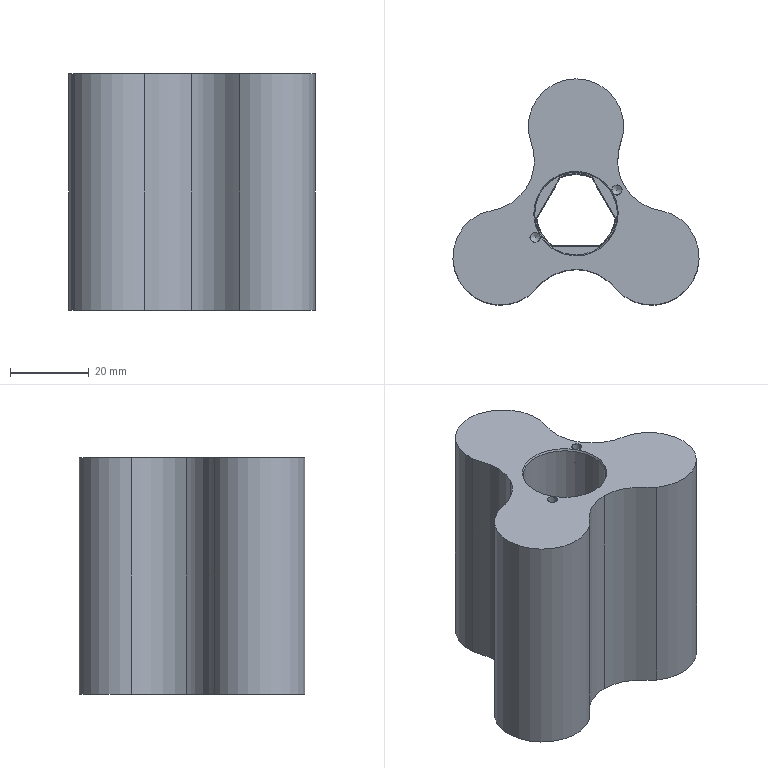NC program | NX | posted with a generic post | part box 62.563 x 57.43 x 60 mm
Whole program:
N10 G17 G21 G94 G90
(DRILLING_COPY_1_COPY_1 , TOOL : ZXZ)
N12 T01 M6
N14 G54
N16 G17 G0 G90 X-10.392 Y-6. S5000 M3
N18 G43 Z30. H1
N20 G94 G81 G98 Z-1. F250. R3.
N22 X10.392 Y6.
N24 G80
N26 G0 X10.392 Y6. Z30.
N28 M5
(DRILLING_COPY_1_COPY_COPY_1 , TOOL : 2.4ZT)
N30 T12 M6
N32 G54
N34 G17 G0 G90 X-10.392 Y-6. S2000 M3
N36 G43 Z30. H12
N38 G94 G83 G98 Z-4.751 F120. Q2. R3.
N40 X10.392 Y6.
N42 G80
N44 G0 X10.392 Y6. Z30.
N46 M5
(DRILLING_COPY_1_COPY_COPY_COPY , TOOL : 2.5JD)
N48 T13 M6
N50 G54
N52 G17 G0 G90 X-10.392 Y-6. S1000 M3
N54 G43 Z30. H13
N56 G94 G85 G98 Z-4. F50. R3.
N58 X10.392 Y6.
N60 G80
N62 G0 X10.392 Y6. Z30.
N64 M5
(ZLEVEL_PROFILE_COPY_1_COPY , TOOL : D12)
N66 T12 M6
N68 G54
N70 G17 G0 G90 X0.209 Y3.338 S3000 M3
N72 G43 Z30. H12
N74 Z-12.2
N76 G94 G1 X0. Y3.7 Z-12.211 F1000.
N78 X-3.204 Y-1.85 Z-12.379
N80 X3.204 Z-12.547
N82 X0. Y3.7 Z-12.714
N84 X-3.204 Y-1.85 Z-12.882
N86 X3.204 Z-13.05
N88 X0. Y3.7 Z-13.218
N90 X-3.204 Y-1.85 Z-13.386
N92 X3.204 Z-13.553
N94 X0. Y3.7 Z-13.721
N96 X-3.204 Y-1.85 Z-13.889
N98 X3.204 Z-14.057
N100 X0. Y3.7 Z-14.225
N102 X-3.204 Y-1.85 Z-14.393
N104 X3.204 Z-14.56
N106 X0. Y3.7 Z-14.728
N108 X-3.204 Y-1.85 Z-14.896
N110 X3.204 Z-15.064
N112 X0. Y3.7 Z-15.232
N114 X-3.204 Y-1.85 Z-15.399
N116 X3.204 F1800.
N118 X0. Y3.7
N120 X-3.204 Y-1.85
N122 X3.143 Z-15.51
N124 X3.023 Y-1.536 Z-15.518
N126 X0.696 Y2.495 Z-15.599
N128 X0. Y3.7
N130 X-3.204 Y-1.85
N132 X3.143 Z-15.71
N134 X3.023 Y-1.536 Z-15.717
N136 X0.696 Y2.495 Z-15.798
N138 X0. Y3.7
N140 X-3.204 Y-1.85
N142 X3.143 Z-15.909
N144 X3.023 Y-1.536 Z-15.916
N146 X0.696 Y2.495 Z-15.998
N148 X0. Y3.7
N150 X-3.204 Y-1.85
N152 X3.143 Z-16.109
N154 X3.023 Y-1.536 Z-16.116
N156 X0.696 Y2.495 Z-16.197
N158 X0. Y3.7
N160 X-3.204 Y-1.85
N162 X3.143 Z-16.308
N164 X3.023 Y-1.536 Z-16.315
N166 X0.696 Y2.495 Z-16.397
N168 X0. Y3.7
N170 X-3.204 Y-1.85
N172 X3.143 Z-16.507
N174 X3.023 Y-1.536 Z-16.515
N176 X0.696 Y2.495 Z-16.596
N178 X0. Y3.7
N180 X-3.204 Y-1.85
N182 X3.143 Z-16.707
N184 X3.023 Y-1.536 Z-16.714
N186 X0.696 Y2.495 Z-16.795
N188 X0. Y3.7
N190 X-3.204 Y-1.85
N192 X3.143 Z-16.906
N194 X3.023 Y-1.536 Z-16.914
N196 X0.696 Y2.495 Z-16.995
N198 X0. Y3.7
N200 X-3.204 Y-1.85
N202 X3.143 Z-17.106
N204 X3.023 Y-1.536 Z-17.113
N206 X0.696 Y2.495 Z-17.194
N208 X0. Y3.7
N210 X-3.204 Y-1.85
N212 X3.143 Z-17.305
N214 X3.023 Y-1.536 Z-17.313
N216 X0.696 Y2.495 Z-17.394
N218 X0. Y3.7
N220 X-3.204 Y-1.85
N222 X3.143 Z-17.505
N224 X3.023 Y-1.536 Z-17.512
N226 X0.696 Y2.495 Z-17.593
N228 X0. Y3.7
N230 X-3.204 Y-1.85
N232 X3.143 Z-17.704
N234 X3.023 Y-1.536 Z-17.711
N236 X0.696 Y2.495 Z-17.793
N238 X0. Y3.7
N240 X-3.204 Y-1.85
N242 X3.143 Z-17.903
N244 X3.023 Y-1.536 Z-17.911
N246 X0.696 Y2.495 Z-17.992
N248 X0. Y3.7
N250 X-3.204 Y-1.85
N252 X3.143 Z-18.103
N254 X3.023 Y-1.536 Z-18.11
N256 X0.696 Y2.495 Z-18.192
N258 X0. Y3.7
N260 X-3.204 Y-1.85
N262 X3.143 Z-18.302
N264 X3.023 Y-1.536 Z-18.31
N266 X0.696 Y2.495 Z-18.391
N268 X0. Y3.7
N270 X-3.204 Y-1.85
N272 X3.143 Z-18.502
N274 X3.023 Y-1.536 Z-18.509
N276 X0.696 Y2.495 Z-18.59
N278 X0. Y3.7
N280 X-3.204 Y-1.85
N282 X3.143 Z-18.701
N284 X3.023 Y-1.536 Z-18.709
N286 X0.696 Y2.495 Z-18.79
N288 X0. Y3.7
N290 X-3.204 Y-1.85
N292 X3.143 Z-18.901
N294 X3.023 Y-1.536 Z-18.908
N296 X0.696 Y2.495 Z-18.989
N298 X0. Y3.7
N300 X-3.204 Y-1.85
N302 X3.143 Z-19.1
N304 X3.023 Y-1.536 Z-19.107
N306 X0.696 Y2.495 Z-19.189
N308 X0. Y3.7
N310 X-3.204 Y-1.85
N312 X3.143 Z-19.299
N314 X3.023 Y-1.536 Z-19.307
N316 X0.696 Y2.495 Z-19.388
N318 X0. Y3.7
N320 X-3.204 Y-1.85
N322 X3.143 Z-19.499
N324 X3.023 Y-1.536 Z-19.506
N326 X0.696 Y2.495 Z-19.588
N328 X0. Y3.7
N330 X-3.204 Y-1.85
N332 X3.143 Z-19.698
N334 X3.023 Y-1.536 Z-19.706
N336 X0.696 Y2.495 Z-19.787
N338 X0. Y3.7
N340 X-3.204 Y-1.85
N342 X3.143 Z-19.898
N344 X3.023 Y-1.536 Z-19.905
N346 X0.696 Y2.495 Z-19.986
N348 X0. Y3.7
N350 X-3.204 Y-1.85
N352 X3.143 Z-20.097
N354 X3.023 Y-1.536 Z-20.105
N356 X0.696 Y2.495 Z-20.186
N358 X0. Y3.7
N360 X-3.204 Y-1.85
N362 X3.143 Z-20.297
N364 X3.023 Y-1.536 Z-20.304
N366 X0.696 Y2.495 Z-20.385
N368 X0. Y3.7
N370 X-3.204 Y-1.85
N372 X3.143 Z-20.496
N374 X3.023 Y-1.536 Z-20.503
N376 X0.696 Y2.495 Z-20.585
N378 X0. Y3.7
N380 X-3.204 Y-1.85
N382 X3.143 Z-20.696
N384 X3.023 Y-1.536 Z-20.703
N386 X0.696 Y2.495 Z-20.784
N388 X0. Y3.7
N390 X-3.204 Y-1.85
N392 X3.143 Z-20.895
N394 X3.023 Y-1.536 Z-20.902
N396 X0.696 Y2.495 Z-20.984
N398 X0. Y3.7
N400 X-3.204 Y-1.85
N402 X3.143 Z-21.094
N404 X3.023 Y-1.536 Z-21.102
N406 X0.696 Y2.495 Z-21.183
N408 X0. Y3.7
N410 X-3.204 Y-1.85
N412 X3.143 Z-21.294
N414 X3.023 Y-1.536 Z-21.301
N416 X0.696 Y2.495 Z-21.382
N418 X0. Y3.7
N420 X-3.204 Y-1.85
N422 X3.143 Z-21.493
N424 X3.023 Y-1.536 Z-21.501
N426 X0.696 Y2.495 Z-21.582
N428 X0. Y3.7
N430 X-3.204 Y-1.85
N432 X3.143 Z-21.693
N434 X3.023 Y-1.536 Z-21.7
N436 X0.696 Y2.495 Z-21.781
N438 X0. Y3.7
N440 X-3.204 Y-1.85
N442 X3.143 Z-21.892
N444 X3.023 Y-1.536 Z-21.9
N446 X0.696 Y2.495 Z-21.981
N448 X0. Y3.7
N450 X-3.204 Y-1.85
N452 X3.143 Z-22.092
N454 X3.023 Y-1.536 Z-22.099
N456 X0.696 Y2.495 Z-22.18
N458 X0. Y3.7
N460 X-3.204 Y-1.85
N462 X3.143 Z-22.291
N464 X3.023 Y-1.536 Z-22.298
N466 X0.696 Y2.495 Z-22.38
N468 X0. Y3.7
N470 X-3.204 Y-1.85
N472 X3.143 Z-22.49
N474 X3.023 Y-1.536 Z-22.498
N476 X0.696 Y2.495 Z-22.579
N478 X0. Y3.7
N480 X-3.204 Y-1.85
N482 X3.143 Z-22.69
N484 X3.023 Y-1.536 Z-22.697
N486 X0.696 Y2.495 Z-22.779
N488 X0. Y3.7
N490 X-3.204 Y-1.85
N492 X3.143 Z-22.889
N494 X3.023 Y-1.536 Z-22.897
N496 X0.696 Y2.495 Z-22.978
N498 X0. Y3.7
N500 X-3.204 Y-1.85
N502 X3.143 Z-23.089
N504 X3.023 Y-1.536 Z-23.096
N506 X0.696 Y2.495 Z-23.177
N508 X0. Y3.7
N510 X-3.204 Y-1.85
N512 X3.143 Z-23.288
N514 X3.023 Y-1.536 Z-23.296
N516 X0.696 Y2.495 Z-23.377
N518 X0. Y3.7
N520 X-3.204 Y-1.85
N522 X3.143 Z-23.488
N524 X3.023 Y-1.536 Z-23.495
N526 X0.696 Y2.495 Z-23.576
N528 X0. Y3.7
N530 X-3.204 Y-1.85
N532 X3.143 Z-23.687
N534 X3.023 Y-1.536 Z-23.694
N536 X0.696 Y2.495 Z-23.776
N538 X0. Y3.7
N540 X-3.204 Y-1.85
N542 X3.143 Z-23.887
N544 X3.023 Y-1.536 Z-23.894
N546 X0.696 Y2.495 Z-23.975
N548 X0. Y3.7
N550 X-3.204 Y-1.85
N552 X3.143 Z-24.086
N554 X3.023 Y-1.536 Z-24.093
N556 X0.696 Y2.495 Z-24.175
N558 X0. Y3.7
N560 X-3.204 Y-1.85
N562 X3.143 Z-24.285
N564 X3.023 Y-1.536 Z-24.293
N566 X0.696 Y2.495 Z-24.374
N568 X0. Y3.7
N570 X-3.204 Y-1.85
N572 X3.143 Z-24.485
N574 X3.023 Y-1.536 Z-24.492
N576 X0.696 Y2.495 Z-24.573
N578 X0. Y3.7
N580 X-3.204 Y-1.85
N582 X3.143 Z-24.684
N584 X3.023 Y-1.536 Z-24.692
N586 X0.696 Y2.495 Z-24.773
N588 X0. Y3.7
N590 X-3.204 Y-1.85
N592 X3.143 Z-24.884
N594 X3.023 Y-1.536 Z-24.891
N596 X0.696 Y2.495 Z-24.972
N598 X0. Y3.7
N600 X-3.204 Y-1.85
N602 X3.143 Z-25.083
N604 X3.023 Y-1.536 Z-25.091
N606 X0.696 Y2.495 Z-25.172
N608 X0. Y3.7
N610 X-3.204 Y-1.85
N612 X3.143 Z-25.283
N614 X3.023 Y-1.536 Z-25.29
N616 X0.696 Y2.495 Z-25.371
N618 X0. Y3.7
N620 X-3.204 Y-1.85
N622 X3.143 Z-25.482
N624 X3.023 Y-1.536 Z-25.489
N626 X0.696 Y2.495 Z-25.571
N628 X0. Y3.7
N630 X-3.204 Y-1.85
N632 X3.143 Z-25.681
N634 X3.023 Y-1.536 Z-25.689
N636 X0.696 Y2.495 Z-25.77
N638 X0. Y3.7
N640 X-3.204 Y-1.85
N642 X3.143 Z-25.881
N644 X3.023 Y-1.536 Z-25.888
N646 X0.696 Y2.495 Z-25.969
N648 X0. Y3.7
N650 X-3.204 Y-1.85
N652 X3.143 Z-26.08
N654 X3.023 Y-1.536 Z-26.088
N656 X0.696 Y2.495 Z-26.169
N658 X0. Y3.7
N660 X-3.204 Y-1.85
N662 X3.143 Z-26.28
N664 X3.023 Y-1.536 Z-26.287
N666 X0.696 Y2.495 Z-26.368
N668 X0. Y3.7
N670 X-3.204 Y-1.85
N672 X3.143 Z-26.479
N674 X3.023 Y-1.536 Z-26.487
N676 X0.696 Y2.495 Z-26.568
N678 X0. Y3.7
N680 X-3.204 Y-1.85
N682 X3.143 Z-26.679
N684 X3.023 Y-1.536 Z-26.686
N686 X0.696 Y2.495 Z-26.767
N688 X0. Y3.7
N690 X-3.204 Y-1.85
N692 X3.143 Z-26.878
N694 X3.023 Y-1.536 Z-26.885
N696 X0.696 Y2.495 Z-26.967
N698 X0. Y3.7
N700 X-3.204 Y-1.85
N702 X3.143 Z-27.077
N704 X3.023 Y-1.536 Z-27.085
N706 X0.696 Y2.495 Z-27.166
N708 X0. Y3.7
N710 X-3.204 Y-1.85
N712 X3.143 Z-27.277
N714 X3.023 Y-1.536 Z-27.284
N716 X0.696 Y2.495 Z-27.366
N718 X0. Y3.7
N720 X-3.204 Y-1.85
N722 X3.143 Z-27.476
N724 X3.023 Y-1.536 Z-27.484
N726 X0.696 Y2.495 Z-27.565
N728 X0. Y3.7
N730 X-3.204 Y-1.85
N732 X3.143 Z-27.676
N734 X3.023 Y-1.536 Z-27.683
N736 X0.696 Y2.495 Z-27.764
N738 X0. Y3.7
N740 X-3.204 Y-1.85
N742 X3.143 Z-27.875
N744 X3.023 Y-1.536 Z-27.883
N746 X0.696 Y2.495 Z-27.964
N748 X0. Y3.7
N750 X-3.204 Y-1.85
N752 X3.143 Z-28.075
N754 X3.023 Y-1.536 Z-28.082
N756 X0.696 Y2.495 Z-28.163
N758 X0. Y3.7
N760 X-3.204 Y-1.85
N762 X3.143 Z-28.274
N764 X3.023 Y-1.536 Z-28.281
N766 X0.696 Y2.495 Z-28.363
N768 X0. Y3.7
N770 X-3.204 Y-1.85
N772 X3.143 Z-28.474
N774 X3.023 Y-1.536 Z-28.481
N776 X0.696 Y2.495 Z-28.562
N778 X0. Y3.7
N780 X-3.204 Y-1.85
N782 X3.143 Z-28.673
N784 X3.023 Y-1.536 Z-28.68
N786 X0.696 Y2.495 Z-28.762
N788 X0. Y3.7
N790 X-3.204 Y-1.85
N792 X3.143 Z-28.872
N794 X3.023 Y-1.536 Z-28.88
N796 X0.696 Y2.495 Z-28.961
N798 X0. Y3.7
N800 X-3.204 Y-1.85
N802 X3.143 Z-29.072
N804 X3.023 Y-1.536 Z-29.079
N806 X0.696 Y2.495 Z-29.16
N808 X0. Y3.7
N810 X-3.204 Y-1.85
N812 X3.143 Z-29.271
N814 X3.023 Y-1.536 Z-29.279
N816 X0.696 Y2.495 Z-29.36
N818 X0. Y3.7
N820 X-3.204 Y-1.85
N822 X3.143 Z-29.471
N824 X3.023 Y-1.536 Z-29.478
N826 X0.696 Y2.495 Z-29.559
N828 X0. Y3.7
N830 X-3.204 Y-1.85
N832 X3.143 Z-29.67
N834 X3.023 Y-1.536 Z-29.678
N836 X0.696 Y2.495 Z-29.759
N838 X0. Y3.7
N840 X-3.204 Y-1.85
N842 X3.143 Z-29.87
N844 X3.023 Y-1.536 Z-29.877
N846 X0.696 Y2.495 Z-29.958
N848 X0. Y3.7
N850 X-3.204 Y-1.85
N852 X3.143 Z-30.069
N854 X3.023 Y-1.536 Z-30.076
N856 X0.696 Y2.495 Z-30.158
N858 X0. Y3.7
N860 X-3.204 Y-1.85
N862 X3.143 Z-30.268
N864 X3.023 Y-1.536 Z-30.276
N866 X0.696 Y2.495 Z-30.357
N868 X0. Y3.7
N870 X-3.204 Y-1.85
N872 X3.143 Z-30.468
N874 X3.023 Y-1.536 Z-30.475
N876 X0.696 Y2.495 Z-30.556
N878 X0. Y3.7
N880 X-3.204 Y-1.85
N882 X3.143 Z-30.667
N884 X3.023 Y-1.536 Z-30.675
N886 X0.696 Y2.495 Z-30.756
N888 X0. Y3.7
N890 X-3.204 Y-1.85
N892 X3.143 Z-30.867
N894 X3.023 Y-1.536 Z-30.874
N896 X0.696 Y2.495 Z-30.955
N898 X0. Y3.7
N900 X-3.204 Y-1.85
N902 X3.143 Z-31.066
N904 X3.023 Y-1.536 Z-31.074
N906 X0.696 Y2.495 Z-31.155
N908 X0. Y3.7
N910 X-3.204 Y-1.85
N912 X3.143 Z-31.266
N914 X3.023 Y-1.536 Z-31.273
N916 X0.696 Y2.495 Z-31.354
N918 X0. Y3.7
N920 X-3.204 Y-1.85
N922 X3.143 Z-31.465
N924 X3.023 Y-1.536 Z-31.472
N926 X0.696 Y2.495 Z-31.554
N928 X0. Y3.7
N930 X-3.204 Y-1.85
N932 X3.143 Z-31.664
N934 X3.023 Y-1.536 Z-31.672
N936 X0.696 Y2.495 Z-31.753
N938 X0. Y3.7
N940 X-3.204 Y-1.85
N942 X3.143 Z-31.864
N944 X3.023 Y-1.536 Z-31.871
N946 X0.696 Y2.495 Z-31.953
N948 X0. Y3.7
N950 X-3.204 Y-1.85
N952 X3.143 Z-32.063
N954 X3.023 Y-1.536 Z-32.071
N956 X0.696 Y2.495 Z-32.152
N958 X0. Y3.7
N960 X-3.204 Y-1.85
N962 X3.143 Z-32.263
N964 X3.023 Y-1.536 Z-32.27
N966 X0.696 Y2.495 Z-32.351
N968 X0. Y3.7
N970 X-3.204 Y-1.85
N972 X3.143 Z-32.462
N974 X3.023 Y-1.536 Z-32.47
N976 X0.696 Y2.495 Z-32.551
N978 X0. Y3.7
N980 X-3.204 Y-1.85
N982 X3.143 Z-32.662
N984 X3.023 Y-1.536 Z-32.669
N986 X0.696 Y2.495 Z-32.75
N988 X0. Y3.7
N990 X-3.204 Y-1.85
N992 X3.143 Z-32.861
N994 X3.023 Y-1.536 Z-32.868
N996 X0.696 Y2.495 Z-32.95
N998 X0. Y3.7
N1000 X-3.204 Y-1.85
N1002 X3.143 Z-33.061
N1004 X3.023 Y-1.536 Z-33.068
N1006 X0.696 Y2.495 Z-33.149
N1008 X0. Y3.7
N1010 X-3.204 Y-1.85
N1012 X3.143 Z-33.26
N1014 X3.023 Y-1.536 Z-33.267
N1016 X0.696 Y2.495 Z-33.349
N1018 X0. Y3.7
N1020 X-3.204 Y-1.85
N1022 X3.143 Z-33.459
N1024 X3.023 Y-1.536 Z-33.467
N1026 X0.696 Y2.495 Z-33.548
N1028 X0. Y3.7
N1030 X-3.204 Y-1.85
N1032 X3.143 Z-33.659
N1034 X3.023 Y-1.536 Z-33.666
N1036 X0.696 Y2.495 Z-33.747
N1038 X0. Y3.7
N1040 X-3.204 Y-1.85
N1042 X3.143 Z-33.858
N1044 X3.023 Y-1.536 Z-33.866
N1046 X0.696 Y2.495 Z-33.947
N1048 X0. Y3.7
N1050 X-3.204 Y-1.85
N1052 X3.143 Z-34.058
N1054 X3.023 Y-1.536 Z-34.065
N1056 X0.696 Y2.495 Z-34.146
N1058 X0. Y3.7
N1060 X-3.204 Y-1.85
N1062 X3.143 Z-34.257
N1064 X3.023 Y-1.536 Z-34.265
N1066 X0.696 Y2.495 Z-34.346
N1068 X0. Y3.7
N1070 X-3.204 Y-1.85
N1072 X3.143 Z-34.457
N1074 X3.023 Y-1.536 Z-34.464
N1076 X0.696 Y2.495 Z-34.545
N1078 X0. Y3.7
N1080 X-3.204 Y-1.85
N1082 X3.143 Z-34.656
N1084 X3.023 Y-1.536 Z-34.663
N1086 X0.696 Y2.495 Z-34.745
N1088 X0. Y3.7
N1090 X-3.204 Y-1.85
N1092 X3.143 Z-34.855
N1094 X3.023 Y-1.536 Z-34.863
N1096 X0.696 Y2.495 Z-34.944
N1098 X0. Y3.7
N1100 X-3.204 Y-1.85
N1102 X3.143 Z-35.055
N1104 X3.023 Y-1.536 Z-35.062
N1106 X0.696 Y2.495 Z-35.144
N1108 X0. Y3.7
N1110 X-3.204 Y-1.85
N1112 X3.143 Z-35.254
N1114 X3.023 Y-1.536 Z-35.262
N1116 X0.696 Y2.495 Z-35.343
N1118 X0. Y3.7
N1120 X-3.204 Y-1.85
N1122 X3.143 Z-35.454
N1124 X3.023 Y-1.536 Z-35.461
N1126 X0.696 Y2.495 Z-35.542
N1128 X0. Y3.7
N1130 X-3.204 Y-1.85
N1132 X3.143 Z-35.653
N1134 X3.023 Y-1.536 Z-35.661
N1136 X0.696 Y2.495 Z-35.742
N1138 X0. Y3.7
N1140 X-3.204 Y-1.85
N1142 X3.143 Z-35.853
N1144 X3.023 Y-1.536 Z-35.86
N1146 X0.696 Y2.495 Z-35.941
N1148 X0. Y3.7
N1150 X-3.204 Y-1.85
N1152 X3.143 Z-36.052
N1154 X3.023 Y-1.536 Z-36.059
N1156 X0.696 Y2.495 Z-36.141
N1158 X0. Y3.7
N1160 X-3.204 Y-1.85
N1162 X3.143 Z-36.251
N1164 X3.023 Y-1.536 Z-36.259
N1166 X0.696 Y2.495 Z-36.34
N1168 X0. Y3.7
N1170 X-3.204 Y-1.85
N1172 X3.143 Z-36.451
N1174 X3.023 Y-1.536 Z-36.458
N1176 X0.696 Y2.495 Z-36.54
N1178 X0. Y3.7
N1180 X-3.204 Y-1.85
N1182 X3.143 Z-36.65
N1184 X3.023 Y-1.536 Z-36.658
N1186 X0.696 Y2.495 Z-36.739
N1188 X0. Y3.7
N1190 X-3.204 Y-1.85
N1192 X3.143 Z-36.85
N1194 X3.023 Y-1.536 Z-36.857
N1196 X0.696 Y2.495 Z-36.938
N1198 X0. Y3.7
N1200 X-3.204 Y-1.85
N1202 X3.143 Z-37.049
N1204 X3.023 Y-1.536 Z-37.057
N1206 X0.696 Y2.495 Z-37.138
N1208 X0. Y3.7
N1210 X-3.204 Y-1.85
N1212 X3.143 Z-37.249
N1214 X3.023 Y-1.536 Z-37.256
N1216 X0.696 Y2.495 Z-37.337
N1218 X0. Y3.7
N1220 X-3.204 Y-1.85
N1222 X3.143 Z-37.448
N1224 X3.023 Y-1.536 Z-37.455
N1226 X0.696 Y2.495 Z-37.537
N1228 X0. Y3.7
N1230 X-3.204 Y-1.85
N1232 X3.143 Z-37.648
N1234 X3.023 Y-1.536 Z-37.655
N1236 X0.696 Y2.495 Z-37.736
N1238 X0. Y3.7
N1240 X-3.204 Y-1.85
N1242 X3.143 Z-37.847
N1244 X3.023 Y-1.536 Z-37.854
N1246 X0.696 Y2.495 Z-37.936
N1248 X0. Y3.7
N1250 X-3.204 Y-1.85
N1252 X3.143 Z-38.046
N1254 X3.023 Y-1.536 Z-38.054
N1256 X0.696 Y2.495 Z-38.135
N1258 X0. Y3.7
N1260 X-3.204 Y-1.85
N1262 X3.143 Z-38.246
N1264 X3.023 Y-1.536 Z-38.253
N1266 X0.696 Y2.495 Z-38.334
N1268 X0. Y3.7
N1270 X-3.204 Y-1.85
N1272 X3.143 Z-38.445
N1274 X3.023 Y-1.536 Z-38.453
N1276 X0.696 Y2.495 Z-38.534
N1278 X0. Y3.7
N1280 X-3.204 Y-1.85
N1282 X3.143 Z-38.645
N1284 X3.023 Y-1.536 Z-38.652
N1286 X0.696 Y2.495 Z-38.733
N1288 X0. Y3.7
N1290 X-3.204 Y-1.85
N1292 X3.143 Z-38.844
N1294 X3.023 Y-1.536 Z-38.852
N1296 X0.696 Y2.495 Z-38.933
N1298 X0. Y3.7
N1300 X-3.204 Y-1.85
N1302 X3.143 Z-39.044
N1304 X3.023 Y-1.536 Z-39.051
N1306 X0.696 Y2.495 Z-39.132
N1308 X0. Y3.7
N1310 X-3.204 Y-1.85
N1312 X3.143 Z-39.243
N1314 X3.023 Y-1.536 Z-39.25
N1316 X0.696 Y2.495 Z-39.332
N1318 X0. Y3.7
N1320 X-3.204 Y-1.85
N1322 X3.143 Z-39.442
N1324 X3.023 Y-1.536 Z-39.45
N1326 X0.696 Y2.495 Z-39.531
N1328 X0. Y3.7
N1330 X-3.204 Y-1.85
N1332 X3.143 Z-39.642
N1334 X3.023 Y-1.536 Z-39.649
N1336 X0.696 Y2.495 Z-39.731
N1338 X0. Y3.7
N1340 X-3.204 Y-1.85
N1342 X3.143 Z-39.841
N1344 X3.023 Y-1.536 Z-39.849
N1346 X0.696 Y2.495 Z-39.93
N1348 X0. Y3.7
N1350 X-3.204 Y-1.85
N1352 X3.143 Z-40.041
N1354 X3.023 Y-1.536 Z-40.048
N1356 X0.696 Y2.495 Z-40.129
N1358 X0. Y3.7
N1360 X-3.204 Y-1.85
N1362 X3.143 Z-40.24
N1364 X3.023 Y-1.536 Z-40.248
N1366 X0.696 Y2.495 Z-40.329
N1368 X0. Y3.7
N1370 X-3.204 Y-1.85
N1372 X3.143 Z-40.44
N1374 X3.023 Y-1.536 Z-40.447
N1376 X0.696 Y2.495 Z-40.528
N1378 X0. Y3.7
N1380 X-3.204 Y-1.85
N1382 X3.143 Z-40.639
N1384 X3.023 Y-1.536 Z-40.646
N1386 X0.696 Y2.495 Z-40.728
N1388 X0. Y3.7
N1390 X-3.204 Y-1.85
N1392 X3.143 Z-40.838
N1394 X3.023 Y-1.536 Z-40.846
N1396 X0.696 Y2.495 Z-40.927
N1398 X0. Y3.7
N1400 X-3.204 Y-1.85
N1402 X3.143 Z-41.038
N1404 X3.023 Y-1.536 Z-41.045
N1406 X0.696 Y2.495 Z-41.127
N1408 X0. Y3.7
N1410 X-3.204 Y-1.85
N1412 X3.143 Z-41.237
N1414 X3.023 Y-1.536 Z-41.245
N1416 X0.696 Y2.495 Z-41.326
N1418 X0. Y3.7
N1420 X-3.204 Y-1.85
N1422 X3.143 Z-41.437
N1424 X3.023 Y-1.536 Z-41.444
N1426 X0.696 Y2.495 Z-41.525
N1428 X0. Y3.7
N1430 X-3.204 Y-1.85
N1432 X3.143 Z-41.636
N1434 X3.023 Y-1.536 Z-41.644
N1436 X0.696 Y2.495 Z-41.725
N1438 X0. Y3.7
N1440 X-3.204 Y-1.85
N1442 X3.143 Z-41.836
N1444 X3.023 Y-1.536 Z-41.843
N1446 X0.696 Y2.495 Z-41.924
N1448 X0. Y3.7
N1450 X-3.204 Y-1.85
N1452 X3.143 Z-42.035
N1454 X3.023 Y-1.536 Z-42.042
N1456 X0.696 Y2.495 Z-42.124
N1458 X0. Y3.7
N1460 X-3.204 Y-1.85
N1462 X3.143 Z-42.235
N1464 X3.023 Y-1.536 Z-42.242
N1466 X0.696 Y2.495 Z-42.323
N1468 X0. Y3.7
N1470 X-3.204 Y-1.85
N1472 X3.143 Z-42.434
N1474 X3.023 Y-1.536 Z-42.441
N1476 X0.696 Y2.495 Z-42.523
N1478 X0. Y3.7
N1480 X-3.204 Y-1.85
N1482 X3.143 Z-42.633
N1484 X3.023 Y-1.536 Z-42.641
N1486 X0.696 Y2.495 Z-42.722
N1488 X0. Y3.7
N1490 X-3.204 Y-1.85
N1492 X3.143 Z-42.833
N1494 X3.023 Y-1.536 Z-42.84
N1496 X0.696 Y2.495 Z-42.921
N1498 X0. Y3.7
N1500 X-3.204 Y-1.85
N1502 X3.143 Z-43.032
N1504 X3.023 Y-1.536 Z-43.04
N1506 X0.696 Y2.495 Z-43.121
N1508 X0. Y3.7
N1510 X-3.204 Y-1.85
N1512 X3.143 Z-43.232
N1514 X3.023 Y-1.536 Z-43.239
N1516 X0.696 Y2.495 Z-43.32
N1518 X0. Y3.7
N1520 X-3.204 Y-1.85
N1522 X3.143 Z-43.431
N1524 X3.023 Y-1.536 Z-43.439
N1526 X0.696 Y2.495 Z-43.52
N1528 X0. Y3.7
N1530 X-3.204 Y-1.85
N1532 X3.143 Z-43.631
N1534 X3.023 Y-1.536 Z-43.638
N1536 X0.696 Y2.495 Z-43.719
N1538 X0. Y3.7
N1540 X-3.204 Y-1.85
N1542 X3.143 Z-43.83
N1544 X3.023 Y-1.536 Z-43.837
N1546 X0.696 Y2.495 Z-43.919
N1548 X0. Y3.7
N1550 X-3.204 Y-1.85
N1552 X3.143 Z-44.029
N1554 X3.023 Y-1.536 Z-44.037
N1556 X0.696 Y2.495 Z-44.118
N1558 X0. Y3.7
N1560 X-3.204 Y-1.85
N1562 X3.143 Z-44.229
N1564 X3.023 Y-1.536 Z-44.236
N1566 X0.696 Y2.495 Z-44.318
N1568 X0. Y3.7
N1570 X-3.204 Y-1.85
N1572 X3.143 Z-44.428
N1574 X3.023 Y-1.536 Z-44.436
N1576 X0.696 Y2.495 Z-44.517
N1578 X0. Y3.7
N1580 X-3.204 Y-1.85
N1582 X3.143 Z-44.628
N1584 X3.023 Y-1.536 Z-44.635
N1586 X0.696 Y2.495 Z-44.716
N1588 X0. Y3.7
N1590 X-3.204 Y-1.85
N1592 X3.143 Z-44.827
N1594 X3.023 Y-1.536 Z-44.835
N1596 X0.696 Y2.495 Z-44.916
N1598 X0. Y3.7
N1600 X-3.204 Y-1.85
N1602 X3.143 Z-45.027
N1604 X3.023 Y-1.536 Z-45.034
N1606 X0.696 Y2.495 Z-45.115
N1608 X0. Y3.7
N1610 X-3.204 Y-1.85
N1612 X3.143 Z-45.226
N1614 X3.023 Y-1.536 Z-45.233
N1616 X0.696 Y2.495 Z-45.315
N1618 X0. Y3.7
N1620 X-3.204 Y-1.85
N1622 X3.143 Z-45.425
N1624 X3.023 Y-1.536 Z-45.433
N1626 X0.696 Y2.495 Z-45.514
N1628 X0. Y3.7
N1630 X-3.204 Y-1.85
N1632 X3.143 Z-45.625
N1634 X3.023 Y-1.536 Z-45.632
N1636 X0.696 Y2.495 Z-45.714
N1638 X0. Y3.7
N1640 X-3.204 Y-1.85
N1642 X3.143 Z-45.824
N1644 X3.023 Y-1.536 Z-45.832
N1646 X0.696 Y2.495 Z-45.913
N1648 X0. Y3.7
N1650 X-3.204 Y-1.85
N1652 X3.143 Z-46.024
N1654 X3.023 Y-1.536 Z-46.031
N1656 X0.696 Y2.495 Z-46.112
N1658 X0. Y3.7
N1660 X-3.204 Y-1.85
N1662 X3.143 Z-46.223
N1664 X3.023 Y-1.536 Z-46.231
N1666 X0.696 Y2.495 Z-46.312
N1668 X0. Y3.7
N1670 X-3.204 Y-1.85
N1672 X3.143 Z-46.423
N1674 X3.023 Y-1.536 Z-46.43
N1676 X0.696 Y2.495 Z-46.511
N1678 X0. Y3.7
N1680 X-3.204 Y-1.85
N1682 X3.143 Z-46.622
N1684 X3.023 Y-1.536 Z-46.629
N1686 X0.696 Y2.495 Z-46.711
N1688 X0. Y3.7
N1690 X-3.204 Y-1.85
N1692 X3.143 Z-46.822
N1694 X3.023 Y-1.536 Z-46.829
N1696 X0.696 Y2.495 Z-46.91
N1698 X0. Y3.7
N1700 X-3.204 Y-1.85
N1702 X3.143 Z-47.021
N1704 X3.023 Y-1.536 Z-47.028
N1706 X0.696 Y2.495 Z-47.11
N1708 X0. Y3.7
N1710 X-3.204 Y-1.85
N1712 X3.143 Z-47.22
N1714 X3.023 Y-1.536 Z-47.228
N1716 X0.696 Y2.495 Z-47.309
N1718 X0. Y3.7
N1720 X-3.204 Y-1.85
N1722 X3.143 Z-47.42
N1724 X3.023 Y-1.536 Z-47.427
N1726 X0.696 Y2.495 Z-47.508
N1728 X0. Y3.7
N1730 X-3.204 Y-1.85
N1732 X3.143 Z-47.619
N1734 X3.023 Y-1.536 Z-47.627
N1736 X0.696 Y2.495 Z-47.708
N1738 X0. Y3.7
N1740 X-3.204 Y-1.85
N1742 X3.143 Z-47.819
N1744 X3.023 Y-1.536 Z-47.826
N1746 X0.696 Y2.495 Z-47.907
N1748 X0. Y3.7
N1750 X-3.204 Y-1.85
N1752 X3.143 Z-48.018
N1754 X3.023 Y-1.536 Z-48.026
N1756 X0.696 Y2.495 Z-48.107
N1758 X0. Y3.7
N1760 X-3.204 Y-1.85
N1762 X3.143 Z-48.218
N1764 X3.023 Y-1.536 Z-48.225
N1766 X0.696 Y2.495 Z-48.306
N1768 X0. Y3.7
N1770 X-3.204 Y-1.85
N1772 X3.143 Z-48.417
N1774 X3.023 Y-1.536 Z-48.424
N1776 X0.696 Y2.495 Z-48.506
N1778 X0. Y3.7
N1780 X-3.204 Y-1.85
N1782 X3.143 Z-48.616
N1784 X3.023 Y-1.536 Z-48.624
N1786 X0.696 Y2.495 Z-48.705
N1788 X0. Y3.7
N1790 X-3.204 Y-1.85
N1792 X3.143 Z-48.816
N1794 X3.023 Y-1.536 Z-48.823
N1796 X0.696 Y2.495 Z-48.905
N1798 X0. Y3.7
N1800 X-3.204 Y-1.85
N1802 X3.143 Z-49.015
N1804 X3.023 Y-1.536 Z-49.023
N1806 X0.696 Y2.495 Z-49.104
N1808 X0. Y3.7
N1810 X-3.204 Y-1.85
N1812 X3.143 Z-49.215
N1814 X3.023 Y-1.536 Z-49.222
N1816 X0.696 Y2.495 Z-49.303
N1818 X0. Y3.7
N1820 X-3.204 Y-1.85
N1822 X3.143 Z-49.414
N1824 X3.023 Y-1.536 Z-49.422
N1826 X0.696 Y2.495 Z-49.503
N1828 X0. Y3.7
N1830 X-3.204 Y-1.85
N1832 X3.143 Z-49.614
N1834 X3.023 Y-1.536 Z-49.621
N1836 X0.696 Y2.495 Z-49.702
N1838 X0. Y3.7
N1840 X-3.204 Y-1.85
N1842 X3.143 Z-49.813
N1844 X3.023 Y-1.536 Z-49.82
N1846 X0.696 Y2.495 Z-49.902
N1848 X0. Y3.7
N1850 X-3.204 Y-1.85
N1852 X3.143 Z-50.012
N1854 X3.023 Y-1.536 Z-50.02
N1856 X0.696 Y2.495 Z-50.101
N1858 X0. Y3.7
N1860 X-3.204 Y-1.85
N1862 X3.143 Z-50.212
N1864 X3.023 Y-1.536 Z-50.219
N1866 X0.696 Y2.495 Z-50.301
N1868 X0. Y3.7
N1870 X-3.204 Y-1.85
N1872 X3.143 Z-50.411
N1874 X3.023 Y-1.536 Z-50.419
N1876 X0.696 Y2.495 Z-50.5
N1878 X0. Y3.7
N1880 X-3.204 Y-1.85
N1882 X3.204
N1884 X0.696 Y2.495
N1886 Z-47.5
N1888 G0 Z30.
(CUTTER_COMP_12_1_COPY , TOOL : D12)
N1890 X-1.205 Y-0.716 S5000
N1892 Z-14.181
N1894 G1 Z-16.181 F1250.
N1896 G41 X-1.299 Y-0.75 D12
N1898 X-2.338 Y-1.35
N1900 G3 X-3.378 Y-1.95 R1.2
N1902 G1 X3.378
N1904 X0. Y3.9
N1906 X-3.378 Y-1.95
N1908 G3 X-2.338 Y-1.35 R1.2
N1910 G1 X-1.299 Y-0.75
N1912 G40
N1914 X-1.222 Y-0.686
N1916 Z-14.181
N1918 G0 Z30.
N1920 X-1.205 Y-0.716
N1922 Z-15.161
N1924 G1 Z-17.161
N1926 G41 X-1.299 Y-0.75
N1928 X-2.338 Y-1.35
N1930 G3 X-3.378 Y-1.95 R1.2
N1932 G1 X3.378
N1934 X0. Y3.9
N1936 X-3.378 Y-1.95
N1938 G3 X-2.338 Y-1.35 R1.2
N1940 G1 X-1.299 Y-0.75
N1942 G40
N1944 X-1.222 Y-0.686
N1946 Z-15.161
N1948 G0 Z30.
N1950 X-1.205 Y-0.716
N1952 Z-16.142
N1954 G1 Z-18.142
N1956 G41 X-1.299 Y-0.75
N1958 X-2.338 Y-1.35
N1960 G3 X-3.378 Y-1.95 R1.2
N1962 G1 X3.378
N1964 X0. Y3.9
N1966 X-3.378 Y-1.95
N1968 G3 X-2.338 Y-1.35 R1.2
N1970 G1 X-1.299 Y-0.75
N1972 G40
N1974 X-1.222 Y-0.686
N1976 Z-16.142
N1978 G0 Z30.
N1980 X-1.205 Y-0.716
N1982 Z-17.122
N1984 G1 Z-19.122
N1986 G41 X-1.299 Y-0.75
N1988 X-2.338 Y-1.35
N1990 G3 X-3.378 Y-1.95 R1.2
N1992 G1 X3.378
N1994 X0. Y3.9
N1996 X-3.378 Y-1.95
N1998 G3 X-2.338 Y-1.35 R1.2
N2000 G1 X-1.299 Y-0.75
N2002 G40
N2004 X-1.222 Y-0.686
N2006 Z-17.122
N2008 G0 Z30.
N2010 X-1.205 Y-0.716
N2012 Z-18.103
N2014 G1 Z-20.103
N2016 G41 X-1.299 Y-0.75
N2018 X-2.338 Y-1.35
N2020 G3 X-3.378 Y-1.95 R1.2
N2022 G1 X3.378
N2024 X0. Y3.9
N2026 X-3.378 Y-1.95
N2028 G3 X-2.338 Y-1.35 R1.2
N2030 G1 X-1.299 Y-0.75
N2032 G40
N2034 X-1.222 Y-0.686
N2036 Z-18.103
N2038 G0 Z30.
N2040 X-1.205 Y-0.716
N2042 Z-19.083
N2044 G1 Z-21.083
N2046 G41 X-1.299 Y-0.75
N2048 X-2.338 Y-1.35
N2050 G3 X-3.378 Y-1.95 R1.2
N2052 G1 X3.378
N2054 X0. Y3.9
N2056 X-3.378 Y-1.95
N2058 G3 X-2.338 Y-1.35 R1.2
N2060 G1 X-1.299 Y-0.75
N2062 G40
N2064 X-1.222 Y-0.686
N2066 Z-19.083
N2068 G0 Z30.
N2070 X-1.205 Y-0.716
N2072 Z-20.064
N2074 G1 Z-22.064
N2076 G41 X-1.299 Y-0.75
N2078 X-2.338 Y-1.35
N2080 G3 X-3.378 Y-1.95 R1.2
N2082 G1 X3.378
N2084 X0. Y3.9
N2086 X-3.378 Y-1.95
N2088 G3 X-2.338 Y-1.35 R1.2
N2090 G1 X-1.299 Y-0.75
N2092 G40
N2094 X-1.222 Y-0.686
N2096 Z-20.064
N2098 G0 Z30.
N2100 X-1.205 Y-0.716
N2102 Z-21.044
N2104 G1 Z-23.044
N2106 G41 X-1.299 Y-0.75
N2108 X-2.338 Y-1.35
N2110 G3 X-3.378 Y-1.95 R1.2
N2112 G1 X3.378
N2114 X0. Y3.9
N2116 X-3.378 Y-1.95
N2118 G3 X-2.338 Y-1.35 R1.2
N2120 G1 X-1.299 Y-0.75
N2122 G40
N2124 X-1.222 Y-0.686
N2126 Z-21.044
N2128 G0 Z30.
N2130 X-1.205 Y-0.716
N2132 Z-22.025
N2134 G1 Z-24.025
N2136 G41 X-1.299 Y-0.75
N2138 X-2.338 Y-1.35
N2140 G3 X-3.378 Y-1.95 R1.2
N2142 G1 X3.378
N2144 X0. Y3.9
N2146 X-3.378 Y-1.95
N2148 G3 X-2.338 Y-1.35 R1.2
N2150 G1 X-1.299 Y-0.75
N2152 G40
N2154 X-1.222 Y-0.686
N2156 Z-22.025
N2158 G0 Z30.
N2160 X-1.205 Y-0.716
N2162 Z-23.006
N2164 G1 Z-25.006
N2166 G41 X-1.299 Y-0.75
N2168 X-2.338 Y-1.35
N2170 G3 X-3.378 Y-1.95 R1.2
N2172 G1 X3.378
N2174 X0. Y3.9
N2176 X-3.378 Y-1.95
N2178 G3 X-2.338 Y-1.35 R1.2
N2180 G1 X-1.299 Y-0.75
N2182 G40
N2184 X-1.222 Y-0.686
N2186 Z-23.006
N2188 G0 Z30.
N2190 X-1.205 Y-0.716
N2192 Z-23.986
N2194 G1 Z-25.986
N2196 G41 X-1.299 Y-0.75
N2198 X-2.338 Y-1.35
N2200 G3 X-3.378 Y-1.95 R1.2
N2202 G1 X3.378
N2204 X0. Y3.9
N2206 X-3.378 Y-1.95
N2208 G3 X-2.338 Y-1.35 R1.2
N2210 G1 X-1.299 Y-0.75
N2212 G40
N2214 X-1.222 Y-0.686
N2216 Z-23.986
N2218 G0 Z30.
N2220 X-1.205 Y-0.716
N2222 Z-24.967
N2224 G1 Z-26.967
N2226 G41 X-1.299 Y-0.75
N2228 X-2.338 Y-1.35
N2230 G3 X-3.378 Y-1.95 R1.2
N2232 G1 X3.378
N2234 X0. Y3.9
N2236 X-3.378 Y-1.95
N2238 G3 X-2.338 Y-1.35 R1.2
N2240 G1 X-1.299 Y-0.75
N2242 G40
N2244 X-1.222 Y-0.686
N2246 Z-24.967
N2248 G0 Z30.
N2250 X-1.205 Y-0.716
N2252 Z-25.947
N2254 G1 Z-27.947
N2256 G41 X-1.299 Y-0.75
N2258 X-2.338 Y-1.35
N2260 G3 X-3.378 Y-1.95 R1.2
N2262 G1 X3.378
N2264 X0. Y3.9
N2266 X-3.378 Y-1.95
N2268 G3 X-2.338 Y-1.35 R1.2
N2270 G1 X-1.299 Y-0.75
N2272 G40
N2274 X-1.222 Y-0.686
N2276 Z-25.947
N2278 G0 Z30.
N2280 X-1.205 Y-0.716
N2282 Z-26.928
N2284 G1 Z-28.928
N2286 G41 X-1.299 Y-0.75
N2288 X-2.338 Y-1.35
N2290 G3 X-3.378 Y-1.95 R1.2
N2292 G1 X3.378
N2294 X0. Y3.9
N2296 X-3.378 Y-1.95
N2298 G3 X-2.338 Y-1.35 R1.2
N2300 G1 X-1.299 Y-0.75
N2302 G40
N2304 X-1.222 Y-0.686
N2306 Z-26.928
N2308 G0 Z30.
N2310 X-1.205 Y-0.716
N2312 Z-27.908
N2314 G1 Z-29.908
N2316 G41 X-1.299 Y-0.75
N2318 X-2.338 Y-1.35
N2320 G3 X-3.378 Y-1.95 R1.2
N2322 G1 X3.378
N2324 X0. Y3.9
N2326 X-3.378 Y-1.95
N2328 G3 X-2.338 Y-1.35 R1.2
N2330 G1 X-1.299 Y-0.75
N2332 G40
N2334 X-1.222 Y-0.686
N2336 Z-27.908
N2338 G0 Z30.
N2340 X-1.205 Y-0.716
N2342 Z-28.889
N2344 G1 Z-30.889
N2346 G41 X-1.299 Y-0.75
N2348 X-2.338 Y-1.35
N2350 G3 X-3.378 Y-1.95 R1.2
N2352 G1 X3.378
N2354 X0. Y3.9
N2356 X-3.378 Y-1.95
N2358 G3 X-2.338 Y-1.35 R1.2
N2360 G1 X-1.299 Y-0.75
N2362 G40
N2364 X-1.222 Y-0.686
N2366 Z-28.889
N2368 G0 Z30.
N2370 X-1.205 Y-0.716
N2372 Z-29.869
N2374 G1 Z-31.869
N2376 G41 X-1.299 Y-0.75
N2378 X-2.338 Y-1.35
N2380 G3 X-3.378 Y-1.95 R1.2
N2382 G1 X3.378
N2384 X0. Y3.9
N2386 X-3.378 Y-1.95
N2388 G3 X-2.338 Y-1.35 R1.2
N2390 G1 X-1.299 Y-0.75
N2392 G40
N2394 X-1.222 Y-0.686
N2396 Z-29.869
N2398 G0 Z30.
N2400 X-1.205 Y-0.716
N2402 Z-30.85
N2404 G1 Z-32.85
N2406 G41 X-1.299 Y-0.75
N2408 X-2.338 Y-1.35
N2410 G3 X-3.378 Y-1.95 R1.2
N2412 G1 X3.378
N2414 X0. Y3.9
N2416 X-3.378 Y-1.95
N2418 G3 X-2.338 Y-1.35 R1.2
N2420 G1 X-1.299 Y-0.75
N2422 G40
N2424 X-1.222 Y-0.686
N2426 Z-30.85
N2428 G0 Z30.
N2430 X-1.205 Y-0.716
N2432 Z-31.831
N2434 G1 Z-33.831
N2436 G41 X-1.299 Y-0.75
N2438 X-2.338 Y-1.35
N2440 G3 X-3.378 Y-1.95 R1.2
N2442 G1 X3.378
N2444 X0. Y3.9
N2446 X-3.378 Y-1.95
N2448 G3 X-2.338 Y-1.35 R1.2
N2450 G1 X-1.299 Y-0.75
N2452 G40
N2454 X-1.222 Y-0.686
N2456 Z-31.831
N2458 G0 Z30.
N2460 X-1.205 Y-0.716
N2462 Z-32.811
N2464 G1 Z-34.811
N2466 G41 X-1.299 Y-0.75
N2468 X-2.338 Y-1.35
N2470 G3 X-3.378 Y-1.95 R1.2
N2472 G1 X3.378
N2474 X0. Y3.9
N2476 X-3.378 Y-1.95
N2478 G3 X-2.338 Y-1.35 R1.2
N2480 G1 X-1.299 Y-0.75
N2482 G40
N2484 X-1.222 Y-0.686
N2486 Z-32.811
N2488 G0 Z30.
N2490 X-1.205 Y-0.716
N2492 Z-33.792
N2494 G1 Z-35.792
N2496 G41 X-1.299 Y-0.75
N2498 X-2.338 Y-1.35
N2500 G3 X-3.378 Y-1.95 R1.2
N2502 G1 X3.378
N2504 X0. Y3.9
N2506 X-3.378 Y-1.95
N2508 G3 X-2.338 Y-1.35 R1.2
N2510 G1 X-1.299 Y-0.75
N2512 G40
N2514 X-1.222 Y-0.686
N2516 Z-33.792
N2518 G0 Z30.
N2520 X-1.205 Y-0.716
N2522 Z-34.772
N2524 G1 Z-36.772
N2526 G41 X-1.299 Y-0.75
N2528 X-2.338 Y-1.35
N2530 G3 X-3.378 Y-1.95 R1.2
N2532 G1 X3.378
N2534 X0. Y3.9
N2536 X-3.378 Y-1.95
N2538 G3 X-2.338 Y-1.35 R1.2
N2540 G1 X-1.299 Y-0.75
N2542 G40
N2544 X-1.222 Y-0.686
N2546 Z-34.772
N2548 G0 Z30.
N2550 X-1.205 Y-0.716
N2552 Z-35.753
N2554 G1 Z-37.753
N2556 G41 X-1.299 Y-0.75
N2558 X-2.338 Y-1.35
N2560 G3 X-3.378 Y-1.95 R1.2
N2562 G1 X3.378
N2564 X0. Y3.9
N2566 X-3.378 Y-1.95
N2568 G3 X-2.338 Y-1.35 R1.2
N2570 G1 X-1.299 Y-0.75
N2572 G40
N2574 X-1.222 Y-0.686
N2576 Z-35.753
N2578 G0 Z30.
N2580 X-1.205 Y-0.716
N2582 Z-36.733
N2584 G1 Z-38.733
N2586 G41 X-1.299 Y-0.75
N2588 X-2.338 Y-1.35
N2590 G3 X-3.378 Y-1.95 R1.2
N2592 G1 X3.378
N2594 X0. Y3.9
N2596 X-3.378 Y-1.95
N2598 G3 X-2.338 Y-1.35 R1.2
N2600 G1 X-1.299 Y-0.75
N2602 G40
N2604 X-1.222 Y-0.686
N2606 Z-36.733
N2608 G0 Z30.
N2610 X-1.205 Y-0.716
N2612 Z-37.714
N2614 G1 Z-39.714
N2616 G41 X-1.299 Y-0.75
N2618 X-2.338 Y-1.35
N2620 G3 X-3.378 Y-1.95 R1.2
N2622 G1 X3.378
N2624 X0. Y3.9
N2626 X-3.378 Y-1.95
N2628 G3 X-2.338 Y-1.35 R1.2
N2630 G1 X-1.299 Y-0.75
N2632 G40
N2634 X-1.222 Y-0.686
N2636 Z-37.714
N2638 G0 Z30.
N2640 X-1.205 Y-0.716
N2642 Z-38.694
N2644 G1 Z-40.694
N2646 G41 X-1.299 Y-0.75
N2648 X-2.338 Y-1.35
N2650 G3 X-3.378 Y-1.95 R1.2
N2652 G1 X3.378
N2654 X0. Y3.9
N2656 X-3.378 Y-1.95
N2658 G3 X-2.338 Y-1.35 R1.2
N2660 G1 X-1.299 Y-0.75
N2662 G40
N2664 X-1.222 Y-0.686
N2666 Z-38.694
N2668 G0 Z30.
N2670 X-1.205 Y-0.716
N2672 Z-39.675
N2674 G1 Z-41.675
N2676 G41 X-1.299 Y-0.75
N2678 X-2.338 Y-1.35
N2680 G3 X-3.378 Y-1.95 R1.2
N2682 G1 X3.378
N2684 X0. Y3.9
N2686 X-3.378 Y-1.95
N2688 G3 X-2.338 Y-1.35 R1.2
N2690 G1 X-1.299 Y-0.75
N2692 G40
N2694 X-1.222 Y-0.686
N2696 Z-39.675
N2698 G0 Z30.
N2700 X-1.205 Y-0.716
N2702 Z-40.656
N2704 G1 Z-42.656
N2706 G41 X-1.299 Y-0.75
N2708 X-2.338 Y-1.35
N2710 G3 X-3.378 Y-1.95 R1.2
N2712 G1 X3.378
N2714 X0. Y3.9
N2716 X-3.378 Y-1.95
N2718 G3 X-2.338 Y-1.35 R1.2
N2720 G1 X-1.299 Y-0.75
N2722 G40
N2724 X-1.222 Y-0.686
N2726 Z-40.656
N2728 G0 Z30.
N2730 X-1.205 Y-0.716
N2732 Z-41.636
N2734 G1 Z-43.636
N2736 G41 X-1.299 Y-0.75
N2738 X-2.338 Y-1.35
N2740 G3 X-3.378 Y-1.95 R1.2
N2742 G1 X3.378
N2744 X0. Y3.9
N2746 X-3.378 Y-1.95
N2748 G3 X-2.338 Y-1.35 R1.2
N2750 G1 X-1.299 Y-0.75
N2752 G40
N2754 X-1.222 Y-0.686
N2756 Z-41.636
N2758 G0 Z30.
N2760 X-1.205 Y-0.716
N2762 Z-42.617
N2764 G1 Z-44.617
N2766 G41 X-1.299 Y-0.75
N2768 X-2.338 Y-1.35
N2770 G3 X-3.378 Y-1.95 R1.2
N2772 G1 X3.378
N2774 X0. Y3.9
N2776 X-3.378 Y-1.95
N2778 G3 X-2.338 Y-1.35 R1.2
N2780 G1 X-1.299 Y-0.75
N2782 G40
N2784 X-1.222 Y-0.686
N2786 Z-42.617
N2788 G0 Z30.
N2790 X-1.205 Y-0.716
N2792 Z-43.597
N2794 G1 Z-45.597
N2796 G41 X-1.299 Y-0.75
N2798 X-2.338 Y-1.35
N2800 G3 X-3.378 Y-1.95 R1.2
N2802 G1 X3.378
N2804 X0. Y3.9
N2806 X-3.378 Y-1.95
N2808 G3 X-2.338 Y-1.35 R1.2
N2810 G1 X-1.299 Y-0.75
N2812 G40
N2814 X-1.222 Y-0.686
N2816 Z-43.597
N2818 G0 Z30.
N2820 X-1.205 Y-0.716
N2822 Z-44.578
N2824 G1 Z-46.578
N2826 G41 X-1.299 Y-0.75
N2828 X-2.338 Y-1.35
N2830 G3 X-3.378 Y-1.95 R1.2
N2832 G1 X3.378
N2834 X0. Y3.9
N2836 X-3.378 Y-1.95
N2838 G3 X-2.338 Y-1.35 R1.2
N2840 G1 X-1.299 Y-0.75
N2842 G40
N2844 X-1.222 Y-0.686
N2846 Z-44.578
N2848 G0 Z30.
N2850 X-1.205 Y-0.716
N2852 Z-45.558
N2854 G1 Z-47.558
N2856 G41 X-1.299 Y-0.75
N2858 X-2.338 Y-1.35
N2860 G3 X-3.378 Y-1.95 R1.2
N2862 G1 X3.378
N2864 X0. Y3.9
N2866 X-3.378 Y-1.95
N2868 G3 X-2.338 Y-1.35 R1.2
N2870 G1 X-1.299 Y-0.75
N2872 G40
N2874 X-1.222 Y-0.686
N2876 Z-45.558
N2878 G0 Z30.
N2880 X-1.205 Y-0.716
N2882 Z-46.539
N2884 G1 Z-48.539
N2886 G41 X-1.299 Y-0.75
N2888 X-2.338 Y-1.35
N2890 G3 X-3.378 Y-1.95 R1.2
N2892 G1 X3.378
N2894 X0. Y3.9
N2896 X-3.378 Y-1.95
N2898 G3 X-2.338 Y-1.35 R1.2
N2900 G1 X-1.299 Y-0.75
N2902 G40
N2904 X-1.222 Y-0.686
N2906 Z-46.539
N2908 G0 Z30.
N2910 X-1.205 Y-0.716
N2912 Z-47.519
N2914 G1 Z-49.519
N2916 G41 X-1.299 Y-0.75
N2918 X-2.338 Y-1.35
N2920 G3 X-3.378 Y-1.95 R1.2
N2922 G1 X3.378
N2924 X0. Y3.9
N2926 X-3.378 Y-1.95
N2928 G3 X-2.338 Y-1.35 R1.2
N2930 G1 X-1.299 Y-0.75
N2932 G40
N2934 X-1.222 Y-0.686
N2936 Z-47.519
N2938 G0 Z30.
N2940 X-1.205 Y-0.716
N2942 Z-48.5
N2944 G1 Z-50.5
N2946 G41 X-1.299 Y-0.75
N2948 X-2.338 Y-1.35
N2950 G3 X-3.378 Y-1.95 R1.2
N2952 G1 X3.378
N2954 X0. Y3.9
N2956 X-3.378 Y-1.95
N2958 G3 X-2.338 Y-1.35 R1.2
N2960 G1 X-1.299 Y-0.75
N2962 G40
N2964 X-1.222 Y-0.686
N2966 Z-48.5
N2968 G0 Z30.
N2970 M5
N2972 M2